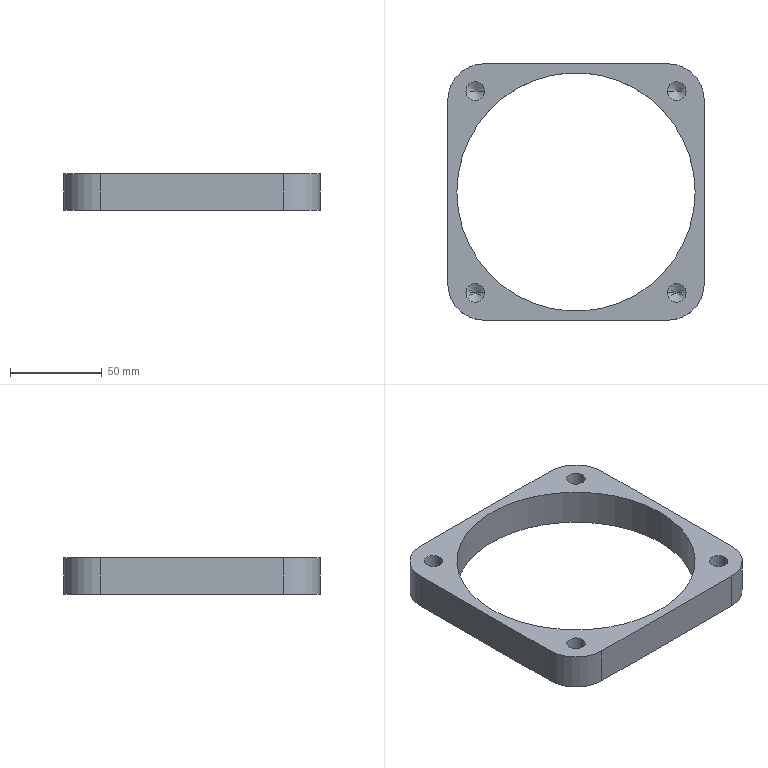Part | SolidWorks | features 3DProfileFeature 1, Extrusion 1, HoleWzd 1 | 1 solid | 28 faces | box 140 x 140 x 20 mm | volume 114105 mm3 | cylinder 14 | cone 8 | plane 6 | commonest cylinder face diameters 10.2 x8 40 x4 130 x2
STEP:
#1=CARTESIAN_POINT('',(9.9,125.,4.));
#2=VERTEX_POINT('',#1);
#3=CARTESIAN_POINT('',(20.1,125.,4.));
#4=VERTEX_POINT('',#3);
#5=CARTESIAN_POINT('',(15.,125.,4.));
#6=DIRECTION('',(0.,0.,1.));
#7=DIRECTION('',(1.,0.,0.));
#8=AXIS2_PLACEMENT_3D('',#5,#6,#7);
#9=CIRCLE('',#8,5.1);
#10=EDGE_CURVE('',#2,#4,#9,.T.);
#11=ORIENTED_EDGE('',*,*,#10,.F.);
#12=CARTESIAN_POINT('',(9.9,125.,20.));
#13=VERTEX_POINT('',#12);
#14=CARTESIAN_POINT('',(9.9,125.,20.));
#15=DIRECTION('',(0.,0.,1.));
#16=VECTOR('',#15,1000.);
#17=LINE('',#14,#16);
#18=EDGE_CURVE('',#2,#13,#17,.T.);
#19=ORIENTED_EDGE('',*,*,#18,.T.);
#20=CARTESIAN_POINT('',(20.1,125.,20.));
#21=VERTEX_POINT('',#20);
#22=CARTESIAN_POINT('',(15.,125.,20.));
#23=DIRECTION('',(0.,0.,1.));
#24=DIRECTION('',(1.,0.,0.));
#25=AXIS2_PLACEMENT_3D('',#22,#23,#24);
#26=CIRCLE('',#25,5.1);
#27=EDGE_CURVE('',#13,#21,#26,.T.);
#28=ORIENTED_EDGE('',*,*,#27,.T.);
#29=CARTESIAN_POINT('',(20.1,125.,20.));
#30=DIRECTION('',(0.,0.,1.));
#31=VECTOR('',#30,1000.);
#32=LINE('',#29,#31);
#33=EDGE_CURVE('',#4,#21,#32,.T.);
#34=ORIENTED_EDGE('',*,*,#33,.F.);
#35=EDGE_LOOP('',(#11,#19,#28,#34));
#36=FACE_OUTER_BOUND('',#35,.T.);
#37=CARTESIAN_POINT('',(15.,125.,20.));
#38=DIRECTION('',(0.,0.,1.));
#39=DIRECTION('',(1.,0.,0.));
#40=AXIS2_PLACEMENT_3D('',#37,#38,#39);
#41=CYLINDRICAL_SURFACE('',#40,5.1);
#42=ADVANCED_FACE('',(#36),#41,.F.);
#43=CARTESIAN_POINT('',(15.,125.,0.9356));
#44=VERTEX_POINT('',#43);
#45=CARTESIAN_POINT('',(20.1,125.,4.));
#46=DIRECTION('',(0.8572,0.,0.515));
#47=VECTOR('',#46,1000.);
#48=LINE('',#45,#47);
#49=EDGE_CURVE('',#44,#4,#48,.T.);
#50=ORIENTED_EDGE('',*,*,#49,.F.);
#51=CARTESIAN_POINT('',(9.9,125.,4.));
#52=DIRECTION('',(-0.8572,0.,0.515));
#53=VECTOR('',#52,1000.);
#54=LINE('',#51,#53);
#55=EDGE_CURVE('',#44,#2,#54,.T.);
#56=ORIENTED_EDGE('',*,*,#55,.T.);
#57=ORIENTED_EDGE('',*,*,#10,.T.);
#58=EDGE_LOOP('',(#50,#56,#57));
#59=FACE_OUTER_BOUND('',#58,.T.);
#60=CARTESIAN_POINT('',(15.,125.,4.));
#61=DIRECTION('',(0.,0.,1.));
#62=DIRECTION('',(1.,0.,0.));
#63=AXIS2_PLACEMENT_3D('',#60,#61,#62);
#64=CONICAL_SURFACE('',#63,5.1,1.03);
#65=ADVANCED_FACE('',(#59),#64,.F.);
#66=CARTESIAN_POINT('',(119.9,125.,4.));
#67=VERTEX_POINT('',#66);
#68=CARTESIAN_POINT('',(130.1,125.,4.));
#69=VERTEX_POINT('',#68);
#70=CARTESIAN_POINT('',(125.,125.,4.));
#71=DIRECTION('',(0.,0.,1.));
#72=DIRECTION('',(1.,0.,0.));
#73=AXIS2_PLACEMENT_3D('',#70,#71,#72);
#74=CIRCLE('',#73,5.1);
#75=EDGE_CURVE('',#67,#69,#74,.T.);
#76=ORIENTED_EDGE('',*,*,#75,.F.);
#77=CARTESIAN_POINT('',(119.9,125.,20.));
#78=VERTEX_POINT('',#77);
#79=CARTESIAN_POINT('',(119.9,125.,20.));
#80=DIRECTION('',(0.,0.,1.));
#81=VECTOR('',#80,1000.);
#82=LINE('',#79,#81);
#83=EDGE_CURVE('',#67,#78,#82,.T.);
#84=ORIENTED_EDGE('',*,*,#83,.T.);
#85=CARTESIAN_POINT('',(130.1,125.,20.));
#86=VERTEX_POINT('',#85);
#87=CARTESIAN_POINT('',(125.,125.,20.));
#88=DIRECTION('',(0.,0.,1.));
#89=DIRECTION('',(1.,0.,0.));
#90=AXIS2_PLACEMENT_3D('',#87,#88,#89);
#91=CIRCLE('',#90,5.1);
#92=EDGE_CURVE('',#78,#86,#91,.T.);
#93=ORIENTED_EDGE('',*,*,#92,.T.);
#94=CARTESIAN_POINT('',(130.1,125.,20.));
#95=DIRECTION('',(0.,0.,1.));
#96=VECTOR('',#95,1000.);
#97=LINE('',#94,#96);
#98=EDGE_CURVE('',#69,#86,#97,.T.);
#99=ORIENTED_EDGE('',*,*,#98,.F.);
#100=EDGE_LOOP('',(#76,#84,#93,#99));
#101=FACE_OUTER_BOUND('',#100,.T.);
#102=CARTESIAN_POINT('',(125.,125.,20.));
#103=DIRECTION('',(0.,0.,1.));
#104=DIRECTION('',(1.,0.,0.));
#105=AXIS2_PLACEMENT_3D('',#102,#103,#104);
#106=CYLINDRICAL_SURFACE('',#105,5.1);
#107=ADVANCED_FACE('',(#101),#106,.F.);
#108=CARTESIAN_POINT('',(125.,125.,0.9356));
#109=VERTEX_POINT('',#108);
#110=CARTESIAN_POINT('',(130.1,125.,4.));
#111=DIRECTION('',(0.8572,0.,0.515));
#112=VECTOR('',#111,1000.);
#113=LINE('',#110,#112);
#114=EDGE_CURVE('',#109,#69,#113,.T.);
#115=ORIENTED_EDGE('',*,*,#114,.F.);
#116=CARTESIAN_POINT('',(119.9,125.,4.));
#117=DIRECTION('',(-0.8572,0.,0.515));
#118=VECTOR('',#117,1000.);
#119=LINE('',#116,#118);
#120=EDGE_CURVE('',#109,#67,#119,.T.);
#121=ORIENTED_EDGE('',*,*,#120,.T.);
#122=ORIENTED_EDGE('',*,*,#75,.T.);
#123=EDGE_LOOP('',(#115,#121,#122));
#124=FACE_OUTER_BOUND('',#123,.T.);
#125=CARTESIAN_POINT('',(125.,125.,4.));
#126=DIRECTION('',(0.,0.,1.));
#127=DIRECTION('',(1.,0.,0.));
#128=AXIS2_PLACEMENT_3D('',#125,#126,#127);
#129=CONICAL_SURFACE('',#128,5.1,1.03);
#130=ADVANCED_FACE('',(#124),#129,.F.);
#131=CARTESIAN_POINT('',(119.9,15.,4.));
#132=VERTEX_POINT('',#131);
#133=CARTESIAN_POINT('',(130.1,15.,4.));
#134=VERTEX_POINT('',#133);
#135=CARTESIAN_POINT('',(125.,15.,4.));
#136=DIRECTION('',(0.,0.,1.));
#137=DIRECTION('',(1.,0.,0.));
#138=AXIS2_PLACEMENT_3D('',#135,#136,#137);
#139=CIRCLE('',#138,5.1);
#140=EDGE_CURVE('',#132,#134,#139,.T.);
#141=ORIENTED_EDGE('',*,*,#140,.F.);
#142=CARTESIAN_POINT('',(119.9,15.,20.));
#143=VERTEX_POINT('',#142);
#144=CARTESIAN_POINT('',(119.9,15.,20.));
#145=DIRECTION('',(0.,0.,1.));
#146=VECTOR('',#145,1000.);
#147=LINE('',#144,#146);
#148=EDGE_CURVE('',#132,#143,#147,.T.);
#149=ORIENTED_EDGE('',*,*,#148,.T.);
#150=CARTESIAN_POINT('',(130.1,15.,20.));
#151=VERTEX_POINT('',#150);
#152=CARTESIAN_POINT('',(125.,15.,20.));
#153=DIRECTION('',(0.,0.,1.));
#154=DIRECTION('',(1.,0.,0.));
#155=AXIS2_PLACEMENT_3D('',#152,#153,#154);
#156=CIRCLE('',#155,5.1);
#157=EDGE_CURVE('',#143,#151,#156,.T.);
#158=ORIENTED_EDGE('',*,*,#157,.T.);
#159=CARTESIAN_POINT('',(130.1,15.,20.));
#160=DIRECTION('',(0.,0.,1.));
#161=VECTOR('',#160,1000.);
#162=LINE('',#159,#161);
#163=EDGE_CURVE('',#134,#151,#162,.T.);
#164=ORIENTED_EDGE('',*,*,#163,.F.);
#165=EDGE_LOOP('',(#141,#149,#158,#164));
#166=FACE_OUTER_BOUND('',#165,.T.);
#167=CARTESIAN_POINT('',(125.,15.,20.));
#168=DIRECTION('',(0.,0.,1.));
#169=DIRECTION('',(1.,0.,0.));
#170=AXIS2_PLACEMENT_3D('',#167,#168,#169);
#171=CYLINDRICAL_SURFACE('',#170,5.1);
#172=ADVANCED_FACE('',(#166),#171,.F.);
#173=CARTESIAN_POINT('',(125.,15.,0.9356));
#174=VERTEX_POINT('',#173);
#175=CARTESIAN_POINT('',(130.1,15.,4.));
#176=DIRECTION('',(0.8572,0.,0.515));
#177=VECTOR('',#176,1000.);
#178=LINE('',#175,#177);
#179=EDGE_CURVE('',#174,#134,#178,.T.);
#180=ORIENTED_EDGE('',*,*,#179,.F.);
#181=CARTESIAN_POINT('',(119.9,15.,4.));
#182=DIRECTION('',(-0.8572,0.,0.515));
#183=VECTOR('',#182,1000.);
#184=LINE('',#181,#183);
#185=EDGE_CURVE('',#174,#132,#184,.T.);
#186=ORIENTED_EDGE('',*,*,#185,.T.);
#187=ORIENTED_EDGE('',*,*,#140,.T.);
#188=EDGE_LOOP('',(#180,#186,#187));
#189=FACE_OUTER_BOUND('',#188,.T.);
#190=CARTESIAN_POINT('',(125.,15.,4.));
#191=DIRECTION('',(0.,0.,1.));
#192=DIRECTION('',(1.,0.,0.));
#193=AXIS2_PLACEMENT_3D('',#190,#191,#192);
#194=CONICAL_SURFACE('',#193,5.1,1.03);
#195=ADVANCED_FACE('',(#189),#194,.F.);
#196=CARTESIAN_POINT('',(9.9,15.,4.));
#197=VERTEX_POINT('',#196);
#198=CARTESIAN_POINT('',(20.1,15.,4.));
#199=VERTEX_POINT('',#198);
#200=CARTESIAN_POINT('',(15.,15.,4.));
#201=DIRECTION('',(0.,0.,1.));
#202=DIRECTION('',(1.,0.,0.));
#203=AXIS2_PLACEMENT_3D('',#200,#201,#202);
#204=CIRCLE('',#203,5.1);
#205=EDGE_CURVE('',#197,#199,#204,.T.);
#206=ORIENTED_EDGE('',*,*,#205,.F.);
#207=CARTESIAN_POINT('',(9.9,15.,20.));
#208=VERTEX_POINT('',#207);
#209=CARTESIAN_POINT('',(9.9,15.,20.));
#210=DIRECTION('',(0.,0.,1.));
#211=VECTOR('',#210,1000.);
#212=LINE('',#209,#211);
#213=EDGE_CURVE('',#197,#208,#212,.T.);
#214=ORIENTED_EDGE('',*,*,#213,.T.);
#215=CARTESIAN_POINT('',(20.1,15.,20.));
#216=VERTEX_POINT('',#215);
#217=CARTESIAN_POINT('',(15.,15.,20.));
#218=DIRECTION('',(0.,0.,1.));
#219=DIRECTION('',(1.,0.,0.));
#220=AXIS2_PLACEMENT_3D('',#217,#218,#219);
#221=CIRCLE('',#220,5.1);
#222=EDGE_CURVE('',#208,#216,#221,.T.);
#223=ORIENTED_EDGE('',*,*,#222,.T.);
#224=CARTESIAN_POINT('',(20.1,15.,20.));
#225=DIRECTION('',(0.,0.,1.));
#226=VECTOR('',#225,1000.);
#227=LINE('',#224,#226);
#228=EDGE_CURVE('',#199,#216,#227,.T.);
#229=ORIENTED_EDGE('',*,*,#228,.F.);
#230=EDGE_LOOP('',(#206,#214,#223,#229));
#231=FACE_OUTER_BOUND('',#230,.T.);
#232=CARTESIAN_POINT('',(15.,15.,20.));
#233=DIRECTION('',(0.,0.,1.));
#234=DIRECTION('',(1.,0.,0.));
#235=AXIS2_PLACEMENT_3D('',#232,#233,#234);
#236=CYLINDRICAL_SURFACE('',#235,5.1);
#237=ADVANCED_FACE('',(#231),#236,.F.);
#238=CARTESIAN_POINT('',(15.,15.,0.9356));
#239=VERTEX_POINT('',#238);
#240=CARTESIAN_POINT('',(20.1,15.,4.));
#241=DIRECTION('',(0.8572,0.,0.515));
#242=VECTOR('',#241,1000.);
#243=LINE('',#240,#242);
#244=EDGE_CURVE('',#239,#199,#243,.T.);
#245=ORIENTED_EDGE('',*,*,#244,.F.);
#246=CARTESIAN_POINT('',(9.9,15.,4.));
#247=DIRECTION('',(-0.8572,0.,0.515));
#248=VECTOR('',#247,1000.);
#249=LINE('',#246,#248);
#250=EDGE_CURVE('',#239,#197,#249,.T.);
#251=ORIENTED_EDGE('',*,*,#250,.T.);
#252=ORIENTED_EDGE('',*,*,#205,.T.);
#253=EDGE_LOOP('',(#245,#251,#252));
#254=FACE_OUTER_BOUND('',#253,.T.);
#255=CARTESIAN_POINT('',(15.,15.,4.));
#256=DIRECTION('',(0.,0.,1.));
#257=DIRECTION('',(1.,0.,0.));
#258=AXIS2_PLACEMENT_3D('',#255,#256,#257);
#259=CONICAL_SURFACE('',#258,5.1,1.03);
#260=ADVANCED_FACE('',(#254),#259,.F.);
#261=CARTESIAN_POINT('',(5.,70.,20.));
#262=VERTEX_POINT('',#261);
#263=CARTESIAN_POINT('',(135.,70.,20.));
#264=VERTEX_POINT('',#263);
#265=CARTESIAN_POINT('',(70.,70.,20.));
#266=DIRECTION('',(0.,0.,1.));
#267=DIRECTION('',(1.,0.,0.));
#268=AXIS2_PLACEMENT_3D('',#265,#266,#267);
#269=CIRCLE('',#268,65.);
#270=EDGE_CURVE('',#262,#264,#269,.T.);
#271=ORIENTED_EDGE('',*,*,#270,.T.);
#272=CARTESIAN_POINT('',(135.,70.,0.));
#273=VERTEX_POINT('',#272);
#274=CARTESIAN_POINT('',(135.,70.,20.));
#275=DIRECTION('',(0.,0.,-1.));
#276=VECTOR('',#275,1000.);
#277=LINE('',#274,#276);
#278=EDGE_CURVE('',#264,#273,#277,.T.);
#279=ORIENTED_EDGE('',*,*,#278,.T.);
#280=CARTESIAN_POINT('',(5.,70.,0.));
#281=VERTEX_POINT('',#280);
#282=CARTESIAN_POINT('',(70.,70.,0.));
#283=DIRECTION('',(0.,0.,1.));
#284=DIRECTION('',(1.,0.,0.));
#285=AXIS2_PLACEMENT_3D('',#282,#283,#284);
#286=CIRCLE('',#285,65.);
#287=EDGE_CURVE('',#281,#273,#286,.T.);
#288=ORIENTED_EDGE('',*,*,#287,.F.);
#289=CARTESIAN_POINT('',(5.,70.,20.));
#290=DIRECTION('',(0.,0.,-1.));
#291=VECTOR('',#290,1000.);
#292=LINE('',#289,#291);
#293=EDGE_CURVE('',#262,#281,#292,.T.);
#294=ORIENTED_EDGE('',*,*,#293,.F.);
#295=EDGE_LOOP('',(#271,#279,#288,#294));
#296=FACE_OUTER_BOUND('',#295,.T.);
#297=CARTESIAN_POINT('',(70.,70.,20.));
#298=DIRECTION('',(0.,0.,-1.));
#299=DIRECTION('',(-1.,0.,0.));
#300=AXIS2_PLACEMENT_3D('',#297,#298,#299);
#301=CYLINDRICAL_SURFACE('',#300,65.);
#302=ADVANCED_FACE('',(#296),#301,.F.);
#303=CARTESIAN_POINT('',(15.,125.,20.));
#304=DIRECTION('',(0.,0.,1.));
#305=DIRECTION('',(1.,0.,0.));
#306=AXIS2_PLACEMENT_3D('',#303,#304,#305);
#307=CIRCLE('',#306,5.1);
#308=EDGE_CURVE('',#21,#13,#307,.T.);
#309=ORIENTED_EDGE('',*,*,#308,.F.);
#310=ORIENTED_EDGE('',*,*,#27,.F.);
#311=EDGE_LOOP('',(#309,#310));
#312=FACE_BOUND('',#311,.T.);
#313=CARTESIAN_POINT('',(125.,125.,20.));
#314=DIRECTION('',(0.,0.,1.));
#315=DIRECTION('',(1.,0.,0.));
#316=AXIS2_PLACEMENT_3D('',#313,#314,#315);
#317=CIRCLE('',#316,5.1);
#318=EDGE_CURVE('',#86,#78,#317,.T.);
#319=ORIENTED_EDGE('',*,*,#318,.F.);
#320=ORIENTED_EDGE('',*,*,#92,.F.);
#321=EDGE_LOOP('',(#319,#320));
#322=FACE_BOUND('',#321,.T.);
#323=CARTESIAN_POINT('',(125.,15.,20.));
#324=DIRECTION('',(0.,0.,1.));
#325=DIRECTION('',(1.,0.,0.));
#326=AXIS2_PLACEMENT_3D('',#323,#324,#325);
#327=CIRCLE('',#326,5.1);
#328=EDGE_CURVE('',#151,#143,#327,.T.);
#329=ORIENTED_EDGE('',*,*,#328,.F.);
#330=ORIENTED_EDGE('',*,*,#157,.F.);
#331=EDGE_LOOP('',(#329,#330));
#332=FACE_BOUND('',#331,.T.);
#333=CARTESIAN_POINT('',(15.,15.,20.));
#334=DIRECTION('',(0.,0.,1.));
#335=DIRECTION('',(1.,0.,0.));
#336=AXIS2_PLACEMENT_3D('',#333,#334,#335);
#337=CIRCLE('',#336,5.1);
#338=EDGE_CURVE('',#216,#208,#337,.T.);
#339=ORIENTED_EDGE('',*,*,#338,.F.);
#340=ORIENTED_EDGE('',*,*,#222,.F.);
#341=EDGE_LOOP('',(#339,#340));
#342=FACE_BOUND('',#341,.T.);
#343=CARTESIAN_POINT('',(0.,20.,20.));
#344=VERTEX_POINT('',#343);
#345=CARTESIAN_POINT('',(20.,0.,20.));
#346=VERTEX_POINT('',#345);
#347=CARTESIAN_POINT('',(20.,20.,20.));
#348=DIRECTION('',(0.,0.,1.));
#349=DIRECTION('',(-1.,0.,0.));
#350=AXIS2_PLACEMENT_3D('',#347,#348,#349);
#351=CIRCLE('',#350,20.);
#352=EDGE_CURVE('',#344,#346,#351,.T.);
#353=ORIENTED_EDGE('',*,*,#352,.T.);
#354=CARTESIAN_POINT('',(120.,0.,20.));
#355=VERTEX_POINT('',#354);
#356=CARTESIAN_POINT('',(20.,0.,20.));
#357=DIRECTION('',(1.,0.,0.));
#358=VECTOR('',#357,1000.);
#359=LINE('',#356,#358);
#360=EDGE_CURVE('',#346,#355,#359,.T.);
#361=ORIENTED_EDGE('',*,*,#360,.T.);
#362=CARTESIAN_POINT('',(140.,20.,20.));
#363=VERTEX_POINT('',#362);
#364=CARTESIAN_POINT('',(120.,20.,20.));
#365=DIRECTION('',(0.,0.,1.));
#366=DIRECTION('',(1.,0.,0.));
#367=AXIS2_PLACEMENT_3D('',#364,#365,#366);
#368=CIRCLE('',#367,20.);
#369=EDGE_CURVE('',#355,#363,#368,.T.);
#370=ORIENTED_EDGE('',*,*,#369,.T.);
#371=CARTESIAN_POINT('',(140.,120.,20.));
#372=VERTEX_POINT('',#371);
#373=CARTESIAN_POINT('',(140.,20.,20.));
#374=DIRECTION('',(0.,1.,0.));
#375=VECTOR('',#374,1000.);
#376=LINE('',#373,#375);
#377=EDGE_CURVE('',#363,#372,#376,.T.);
#378=ORIENTED_EDGE('',*,*,#377,.T.);
#379=CARTESIAN_POINT('',(120.,140.,20.));
#380=VERTEX_POINT('',#379);
#381=CARTESIAN_POINT('',(120.,120.,20.));
#382=DIRECTION('',(0.,0.,1.));
#383=DIRECTION('',(-1.,0.,0.));
#384=AXIS2_PLACEMENT_3D('',#381,#382,#383);
#385=CIRCLE('',#384,20.);
#386=EDGE_CURVE('',#372,#380,#385,.T.);
#387=ORIENTED_EDGE('',*,*,#386,.T.);
#388=CARTESIAN_POINT('',(20.,140.,20.));
#389=VERTEX_POINT('',#388);
#390=CARTESIAN_POINT('',(20.,140.,20.));
#391=DIRECTION('',(-1.,0.,0.));
#392=VECTOR('',#391,1000.);
#393=LINE('',#390,#392);
#394=EDGE_CURVE('',#380,#389,#393,.T.);
#395=ORIENTED_EDGE('',*,*,#394,.T.);
#396=CARTESIAN_POINT('',(0.,120.,20.));
#397=VERTEX_POINT('',#396);
#398=CARTESIAN_POINT('',(20.,120.,20.));
#399=DIRECTION('',(0.,0.,1.));
#400=DIRECTION('',(-1.,0.,0.));
#401=AXIS2_PLACEMENT_3D('',#398,#399,#400);
#402=CIRCLE('',#401,20.);
#403=EDGE_CURVE('',#389,#397,#402,.T.);
#404=ORIENTED_EDGE('',*,*,#403,.T.);
#405=CARTESIAN_POINT('',(0.,20.,20.));
#406=DIRECTION('',(0.,-1.,0.));
#407=VECTOR('',#406,1000.);
#408=LINE('',#405,#407);
#409=EDGE_CURVE('',#397,#344,#408,.T.);
#410=ORIENTED_EDGE('',*,*,#409,.T.);
#411=EDGE_LOOP('',(#353,#361,#370,#378,#387,#395,#404,#410));
#412=FACE_OUTER_BOUND('',#411,.T.);
#413=ORIENTED_EDGE('',*,*,#270,.F.);
#414=CARTESIAN_POINT('',(70.,70.,20.));
#415=DIRECTION('',(0.,0.,1.));
#416=DIRECTION('',(1.,0.,0.));
#417=AXIS2_PLACEMENT_3D('',#414,#415,#416);
#418=CIRCLE('',#417,65.);
#419=EDGE_CURVE('',#264,#262,#418,.T.);
#420=ORIENTED_EDGE('',*,*,#419,.F.);
#421=EDGE_LOOP('',(#413,#420));
#422=FACE_BOUND('',#421,.T.);
#423=CARTESIAN_POINT('',(20.,20.,20.));
#424=DIRECTION('',(0.,0.,-1.));
#425=DIRECTION('',(-1.,0.,0.));
#426=AXIS2_PLACEMENT_3D('',#423,#424,#425);
#427=PLANE('',#426);
#428=ADVANCED_FACE('',(#312,#322,#332,#342,#412,#422),#427,.F.);
#429=CARTESIAN_POINT('',(0.,20.,0.));
#430=VERTEX_POINT('',#429);
#431=CARTESIAN_POINT('',(20.,0.,0.));
#432=VERTEX_POINT('',#431);
#433=CARTESIAN_POINT('',(20.,20.,0.));
#434=DIRECTION('',(0.,0.,1.));
#435=DIRECTION('',(-1.,0.,0.));
#436=AXIS2_PLACEMENT_3D('',#433,#434,#435);
#437=CIRCLE('',#436,20.);
#438=EDGE_CURVE('',#430,#432,#437,.T.);
#439=ORIENTED_EDGE('',*,*,#438,.F.);
#440=CARTESIAN_POINT('',(0.,120.,0.));
#441=VERTEX_POINT('',#440);
#442=CARTESIAN_POINT('',(0.,20.,0.));
#443=DIRECTION('',(0.,-1.,0.));
#444=VECTOR('',#443,1000.);
#445=LINE('',#442,#444);
#446=EDGE_CURVE('',#441,#430,#445,.T.);
#447=ORIENTED_EDGE('',*,*,#446,.F.);
#448=CARTESIAN_POINT('',(20.,140.,0.));
#449=VERTEX_POINT('',#448);
#450=CARTESIAN_POINT('',(20.,120.,0.));
#451=DIRECTION('',(0.,0.,1.));
#452=DIRECTION('',(-1.,0.,0.));
#453=AXIS2_PLACEMENT_3D('',#450,#451,#452);
#454=CIRCLE('',#453,20.);
#455=EDGE_CURVE('',#449,#441,#454,.T.);
#456=ORIENTED_EDGE('',*,*,#455,.F.);
#457=CARTESIAN_POINT('',(120.,140.,0.));
#458=VERTEX_POINT('',#457);
#459=CARTESIAN_POINT('',(20.,140.,0.));
#460=DIRECTION('',(-1.,0.,0.));
#461=VECTOR('',#460,1000.);
#462=LINE('',#459,#461);
#463=EDGE_CURVE('',#458,#449,#462,.T.);
#464=ORIENTED_EDGE('',*,*,#463,.F.);
#465=CARTESIAN_POINT('',(140.,120.,0.));
#466=VERTEX_POINT('',#465);
#467=CARTESIAN_POINT('',(120.,120.,0.));
#468=DIRECTION('',(0.,0.,1.));
#469=DIRECTION('',(-1.,0.,0.));
#470=AXIS2_PLACEMENT_3D('',#467,#468,#469);
#471=CIRCLE('',#470,20.);
#472=EDGE_CURVE('',#466,#458,#471,.T.);
#473=ORIENTED_EDGE('',*,*,#472,.F.);
#474=CARTESIAN_POINT('',(140.,20.,0.));
#475=VERTEX_POINT('',#474);
#476=CARTESIAN_POINT('',(140.,20.,0.));
#477=DIRECTION('',(0.,1.,0.));
#478=VECTOR('',#477,1000.);
#479=LINE('',#476,#478);
#480=EDGE_CURVE('',#475,#466,#479,.T.);
#481=ORIENTED_EDGE('',*,*,#480,.F.);
#482=CARTESIAN_POINT('',(120.,0.,0.));
#483=VERTEX_POINT('',#482);
#484=CARTESIAN_POINT('',(120.,20.,0.));
#485=DIRECTION('',(0.,0.,1.));
#486=DIRECTION('',(1.,0.,0.));
#487=AXIS2_PLACEMENT_3D('',#484,#485,#486);
#488=CIRCLE('',#487,20.);
#489=EDGE_CURVE('',#483,#475,#488,.T.);
#490=ORIENTED_EDGE('',*,*,#489,.F.);
#491=CARTESIAN_POINT('',(20.,0.,0.));
#492=DIRECTION('',(1.,0.,0.));
#493=VECTOR('',#492,1000.);
#494=LINE('',#491,#493);
#495=EDGE_CURVE('',#432,#483,#494,.T.);
#496=ORIENTED_EDGE('',*,*,#495,.F.);
#497=EDGE_LOOP('',(#439,#447,#456,#464,#473,#481,#490,#496));
#498=FACE_OUTER_BOUND('',#497,.T.);
#499=ORIENTED_EDGE('',*,*,#287,.T.);
#500=CARTESIAN_POINT('',(70.,70.,0.));
#501=DIRECTION('',(0.,0.,1.));
#502=DIRECTION('',(1.,0.,0.));
#503=AXIS2_PLACEMENT_3D('',#500,#501,#502);
#504=CIRCLE('',#503,65.);
#505=EDGE_CURVE('',#273,#281,#504,.T.);
#506=ORIENTED_EDGE('',*,*,#505,.T.);
#507=EDGE_LOOP('',(#499,#506));
#508=FACE_BOUND('',#507,.T.);
#509=CARTESIAN_POINT('',(20.,20.,0.));
#510=DIRECTION('',(0.,0.,-1.));
#511=DIRECTION('',(-1.,0.,0.));
#512=AXIS2_PLACEMENT_3D('',#509,#510,#511);
#513=PLANE('',#512);
#514=ADVANCED_FACE('',(#498,#508),#513,.T.);
#515=ORIENTED_EDGE('',*,*,#438,.T.);
#516=CARTESIAN_POINT('',(20.,0.,20.));
#517=DIRECTION('',(0.,0.,-1.));
#518=VECTOR('',#517,1000.);
#519=LINE('',#516,#518);
#520=EDGE_CURVE('',#346,#432,#519,.T.);
#521=ORIENTED_EDGE('',*,*,#520,.F.);
#522=ORIENTED_EDGE('',*,*,#352,.F.);
#523=CARTESIAN_POINT('',(0.,20.,20.));
#524=DIRECTION('',(0.,0.,-1.));
#525=VECTOR('',#524,1000.);
#526=LINE('',#523,#525);
#527=EDGE_CURVE('',#344,#430,#526,.T.);
#528=ORIENTED_EDGE('',*,*,#527,.T.);
#529=EDGE_LOOP('',(#515,#521,#522,#528));
#530=FACE_OUTER_BOUND('',#529,.T.);
#531=CARTESIAN_POINT('',(20.,20.,20.));
#532=DIRECTION('',(0.,0.,-1.));
#533=DIRECTION('',(-1.,0.,0.));
#534=AXIS2_PLACEMENT_3D('',#531,#532,#533);
#535=CYLINDRICAL_SURFACE('',#534,20.);
#536=ADVANCED_FACE('',(#530),#535,.T.);
#537=ORIENTED_EDGE('',*,*,#495,.T.);
#538=CARTESIAN_POINT('',(120.,0.,20.));
#539=DIRECTION('',(0.,0.,-1.));
#540=VECTOR('',#539,1000.);
#541=LINE('',#538,#540);
#542=EDGE_CURVE('',#355,#483,#541,.T.);
#543=ORIENTED_EDGE('',*,*,#542,.F.);
#544=ORIENTED_EDGE('',*,*,#360,.F.);
#545=ORIENTED_EDGE('',*,*,#520,.T.);
#546=EDGE_LOOP('',(#537,#543,#544,#545));
#547=FACE_OUTER_BOUND('',#546,.T.);
#548=CARTESIAN_POINT('',(20.,0.,20.));
#549=DIRECTION('',(0.,1.,0.));
#550=DIRECTION('',(0.,0.,1.));
#551=AXIS2_PLACEMENT_3D('',#548,#549,#550);
#552=PLANE('',#551);
#553=ADVANCED_FACE('',(#547),#552,.F.);
#554=ORIENTED_EDGE('',*,*,#489,.T.);
#555=CARTESIAN_POINT('',(140.,20.,20.));
#556=DIRECTION('',(0.,0.,-1.));
#557=VECTOR('',#556,1000.);
#558=LINE('',#555,#557);
#559=EDGE_CURVE('',#363,#475,#558,.T.);
#560=ORIENTED_EDGE('',*,*,#559,.F.);
#561=ORIENTED_EDGE('',*,*,#369,.F.);
#562=ORIENTED_EDGE('',*,*,#542,.T.);
#563=EDGE_LOOP('',(#554,#560,#561,#562));
#564=FACE_OUTER_BOUND('',#563,.T.);
#565=CARTESIAN_POINT('',(120.,20.,20.));
#566=DIRECTION('',(0.,0.,-1.));
#567=DIRECTION('',(-1.,0.,0.));
#568=AXIS2_PLACEMENT_3D('',#565,#566,#567);
#569=CYLINDRICAL_SURFACE('',#568,20.);
#570=ADVANCED_FACE('',(#564),#569,.T.);
#571=ORIENTED_EDGE('',*,*,#480,.T.);
#572=CARTESIAN_POINT('',(140.,120.,20.));
#573=DIRECTION('',(0.,0.,-1.));
#574=VECTOR('',#573,1000.);
#575=LINE('',#572,#574);
#576=EDGE_CURVE('',#372,#466,#575,.T.);
#577=ORIENTED_EDGE('',*,*,#576,.F.);
#578=ORIENTED_EDGE('',*,*,#377,.F.);
#579=ORIENTED_EDGE('',*,*,#559,.T.);
#580=EDGE_LOOP('',(#571,#577,#578,#579));
#581=FACE_OUTER_BOUND('',#580,.T.);
#582=CARTESIAN_POINT('',(140.,20.,20.));
#583=DIRECTION('',(-1.,0.,0.));
#584=DIRECTION('',(0.,0.,1.));
#585=AXIS2_PLACEMENT_3D('',#582,#583,#584);
#586=PLANE('',#585);
#587=ADVANCED_FACE('',(#581),#586,.F.);
#588=ORIENTED_EDGE('',*,*,#472,.T.);
#589=CARTESIAN_POINT('',(120.,140.,20.));
#590=DIRECTION('',(0.,0.,-1.));
#591=VECTOR('',#590,1000.);
#592=LINE('',#589,#591);
#593=EDGE_CURVE('',#380,#458,#592,.T.);
#594=ORIENTED_EDGE('',*,*,#593,.F.);
#595=ORIENTED_EDGE('',*,*,#386,.F.);
#596=ORIENTED_EDGE('',*,*,#576,.T.);
#597=EDGE_LOOP('',(#588,#594,#595,#596));
#598=FACE_OUTER_BOUND('',#597,.T.);
#599=CARTESIAN_POINT('',(120.,120.,20.));
#600=DIRECTION('',(0.,0.,-1.));
#601=DIRECTION('',(-1.,0.,0.));
#602=AXIS2_PLACEMENT_3D('',#599,#600,#601);
#603=CYLINDRICAL_SURFACE('',#602,20.);
#604=ADVANCED_FACE('',(#598),#603,.T.);
#605=ORIENTED_EDGE('',*,*,#463,.T.);
#606=CARTESIAN_POINT('',(20.,140.,20.));
#607=DIRECTION('',(0.,0.,-1.));
#608=VECTOR('',#607,1000.);
#609=LINE('',#606,#608);
#610=EDGE_CURVE('',#389,#449,#609,.T.);
#611=ORIENTED_EDGE('',*,*,#610,.F.);
#612=ORIENTED_EDGE('',*,*,#394,.F.);
#613=ORIENTED_EDGE('',*,*,#593,.T.);
#614=EDGE_LOOP('',(#605,#611,#612,#613));
#615=FACE_OUTER_BOUND('',#614,.T.);
#616=CARTESIAN_POINT('',(20.,140.,20.));
#617=DIRECTION('',(0.,-1.,0.));
#618=DIRECTION('',(0.,0.,-1.));
#619=AXIS2_PLACEMENT_3D('',#616,#617,#618);
#620=PLANE('',#619);
#621=ADVANCED_FACE('',(#615),#620,.F.);
#622=ORIENTED_EDGE('',*,*,#455,.T.);
#623=CARTESIAN_POINT('',(0.,120.,20.));
#624=DIRECTION('',(0.,0.,-1.));
#625=VECTOR('',#624,1000.);
#626=LINE('',#623,#625);
#627=EDGE_CURVE('',#397,#441,#626,.T.);
#628=ORIENTED_EDGE('',*,*,#627,.F.);
#629=ORIENTED_EDGE('',*,*,#403,.F.);
#630=ORIENTED_EDGE('',*,*,#610,.T.);
#631=EDGE_LOOP('',(#622,#628,#629,#630));
#632=FACE_OUTER_BOUND('',#631,.T.);
#633=CARTESIAN_POINT('',(20.,120.,20.));
#634=DIRECTION('',(0.,0.,-1.));
#635=DIRECTION('',(-1.,0.,0.));
#636=AXIS2_PLACEMENT_3D('',#633,#634,#635);
#637=CYLINDRICAL_SURFACE('',#636,20.);
#638=ADVANCED_FACE('',(#632),#637,.T.);
#639=ORIENTED_EDGE('',*,*,#446,.T.);
#640=ORIENTED_EDGE('',*,*,#527,.F.);
#641=ORIENTED_EDGE('',*,*,#409,.F.);
#642=ORIENTED_EDGE('',*,*,#627,.T.);
#643=EDGE_LOOP('',(#639,#640,#641,#642));
#644=FACE_OUTER_BOUND('',#643,.T.);
#645=CARTESIAN_POINT('',(0.,20.,20.));
#646=DIRECTION('',(1.,0.,0.));
#647=DIRECTION('',(0.,0.,-1.));
#648=AXIS2_PLACEMENT_3D('',#645,#646,#647);
#649=PLANE('',#648);
#650=ADVANCED_FACE('',(#644),#649,.F.);
#651=ORIENTED_EDGE('',*,*,#278,.F.);
#652=ORIENTED_EDGE('',*,*,#419,.T.);
#653=ORIENTED_EDGE('',*,*,#293,.T.);
#654=ORIENTED_EDGE('',*,*,#505,.F.);
#655=EDGE_LOOP('',(#651,#652,#653,#654));
#656=FACE_OUTER_BOUND('',#655,.T.);
#657=CARTESIAN_POINT('',(70.,70.,20.));
#658=DIRECTION('',(0.,0.,-1.));
#659=DIRECTION('',(-1.,0.,0.));
#660=AXIS2_PLACEMENT_3D('',#657,#658,#659);
#661=CYLINDRICAL_SURFACE('',#660,65.);
#662=ADVANCED_FACE('',(#656),#661,.F.);
#663=ORIENTED_EDGE('',*,*,#250,.F.);
#664=ORIENTED_EDGE('',*,*,#244,.T.);
#665=CARTESIAN_POINT('',(15.,15.,4.));
#666=DIRECTION('',(0.,0.,1.));
#667=DIRECTION('',(1.,0.,0.));
#668=AXIS2_PLACEMENT_3D('',#665,#666,#667);
#669=CIRCLE('',#668,5.1);
#670=EDGE_CURVE('',#199,#197,#669,.T.);
#671=ORIENTED_EDGE('',*,*,#670,.T.);
#672=EDGE_LOOP('',(#663,#664,#671));
#673=FACE_OUTER_BOUND('',#672,.T.);
#674=CARTESIAN_POINT('',(15.,15.,4.));
#675=DIRECTION('',(0.,0.,1.));
#676=DIRECTION('',(1.,0.,0.));
#677=AXIS2_PLACEMENT_3D('',#674,#675,#676);
#678=CONICAL_SURFACE('',#677,5.1,1.03);
#679=ADVANCED_FACE('',(#673),#678,.F.);
#680=ORIENTED_EDGE('',*,*,#213,.F.);
#681=ORIENTED_EDGE('',*,*,#670,.F.);
#682=ORIENTED_EDGE('',*,*,#228,.T.);
#683=ORIENTED_EDGE('',*,*,#338,.T.);
#684=EDGE_LOOP('',(#680,#681,#682,#683));
#685=FACE_OUTER_BOUND('',#684,.T.);
#686=CARTESIAN_POINT('',(15.,15.,20.));
#687=DIRECTION('',(0.,0.,1.));
#688=DIRECTION('',(1.,0.,0.));
#689=AXIS2_PLACEMENT_3D('',#686,#687,#688);
#690=CYLINDRICAL_SURFACE('',#689,5.1);
#691=ADVANCED_FACE('',(#685),#690,.F.);
#692=ORIENTED_EDGE('',*,*,#185,.F.);
#693=ORIENTED_EDGE('',*,*,#179,.T.);
#694=CARTESIAN_POINT('',(125.,15.,4.));
#695=DIRECTION('',(0.,0.,1.));
#696=DIRECTION('',(1.,0.,0.));
#697=AXIS2_PLACEMENT_3D('',#694,#695,#696);
#698=CIRCLE('',#697,5.1);
#699=EDGE_CURVE('',#134,#132,#698,.T.);
#700=ORIENTED_EDGE('',*,*,#699,.T.);
#701=EDGE_LOOP('',(#692,#693,#700));
#702=FACE_OUTER_BOUND('',#701,.T.);
#703=CARTESIAN_POINT('',(125.,15.,4.));
#704=DIRECTION('',(0.,0.,1.));
#705=DIRECTION('',(1.,0.,0.));
#706=AXIS2_PLACEMENT_3D('',#703,#704,#705);
#707=CONICAL_SURFACE('',#706,5.1,1.03);
#708=ADVANCED_FACE('',(#702),#707,.F.);
#709=ORIENTED_EDGE('',*,*,#148,.F.);
#710=ORIENTED_EDGE('',*,*,#699,.F.);
#711=ORIENTED_EDGE('',*,*,#163,.T.);
#712=ORIENTED_EDGE('',*,*,#328,.T.);
#713=EDGE_LOOP('',(#709,#710,#711,#712));
#714=FACE_OUTER_BOUND('',#713,.T.);
#715=CARTESIAN_POINT('',(125.,15.,20.));
#716=DIRECTION('',(0.,0.,1.));
#717=DIRECTION('',(1.,0.,0.));
#718=AXIS2_PLACEMENT_3D('',#715,#716,#717);
#719=CYLINDRICAL_SURFACE('',#718,5.1);
#720=ADVANCED_FACE('',(#714),#719,.F.);
#721=ORIENTED_EDGE('',*,*,#120,.F.);
#722=ORIENTED_EDGE('',*,*,#114,.T.);
#723=CARTESIAN_POINT('',(125.,125.,4.));
#724=DIRECTION('',(0.,0.,1.));
#725=DIRECTION('',(1.,0.,0.));
#726=AXIS2_PLACEMENT_3D('',#723,#724,#725);
#727=CIRCLE('',#726,5.1);
#728=EDGE_CURVE('',#69,#67,#727,.T.);
#729=ORIENTED_EDGE('',*,*,#728,.T.);
#730=EDGE_LOOP('',(#721,#722,#729));
#731=FACE_OUTER_BOUND('',#730,.T.);
#732=CARTESIAN_POINT('',(125.,125.,4.));
#733=DIRECTION('',(0.,0.,1.));
#734=DIRECTION('',(1.,0.,0.));
#735=AXIS2_PLACEMENT_3D('',#732,#733,#734);
#736=CONICAL_SURFACE('',#735,5.1,1.03);
#737=ADVANCED_FACE('',(#731),#736,.F.);
#738=ORIENTED_EDGE('',*,*,#83,.F.);
#739=ORIENTED_EDGE('',*,*,#728,.F.);
#740=ORIENTED_EDGE('',*,*,#98,.T.);
#741=ORIENTED_EDGE('',*,*,#318,.T.);
#742=EDGE_LOOP('',(#738,#739,#740,#741));
#743=FACE_OUTER_BOUND('',#742,.T.);
#744=CARTESIAN_POINT('',(125.,125.,20.));
#745=DIRECTION('',(0.,0.,1.));
#746=DIRECTION('',(1.,0.,0.));
#747=AXIS2_PLACEMENT_3D('',#744,#745,#746);
#748=CYLINDRICAL_SURFACE('',#747,5.1);
#749=ADVANCED_FACE('',(#743),#748,.F.);
#750=ORIENTED_EDGE('',*,*,#55,.F.);
#751=ORIENTED_EDGE('',*,*,#49,.T.);
#752=CARTESIAN_POINT('',(15.,125.,4.));
#753=DIRECTION('',(0.,0.,1.));
#754=DIRECTION('',(1.,0.,0.));
#755=AXIS2_PLACEMENT_3D('',#752,#753,#754);
#756=CIRCLE('',#755,5.1);
#757=EDGE_CURVE('',#4,#2,#756,.T.);
#758=ORIENTED_EDGE('',*,*,#757,.T.);
#759=EDGE_LOOP('',(#750,#751,#758));
#760=FACE_OUTER_BOUND('',#759,.T.);
#761=CARTESIAN_POINT('',(15.,125.,4.));
#762=DIRECTION('',(0.,0.,1.));
#763=DIRECTION('',(1.,0.,0.));
#764=AXIS2_PLACEMENT_3D('',#761,#762,#763);
#765=CONICAL_SURFACE('',#764,5.1,1.03);
#766=ADVANCED_FACE('',(#760),#765,.F.);
#767=ORIENTED_EDGE('',*,*,#18,.F.);
#768=ORIENTED_EDGE('',*,*,#757,.F.);
#769=ORIENTED_EDGE('',*,*,#33,.T.);
#770=ORIENTED_EDGE('',*,*,#308,.T.);
#771=EDGE_LOOP('',(#767,#768,#769,#770));
#772=FACE_OUTER_BOUND('',#771,.T.);
#773=CARTESIAN_POINT('',(15.,125.,20.));
#774=DIRECTION('',(0.,0.,1.));
#775=DIRECTION('',(1.,0.,0.));
#776=AXIS2_PLACEMENT_3D('',#773,#774,#775);
#777=CYLINDRICAL_SURFACE('',#776,5.1);
#778=ADVANCED_FACE('',(#772),#777,.F.);
#779=CLOSED_SHELL('',(#42,#65,#107,#130,#172,#195,#237,#260,#302,#428,#514,#536,#553,#570,#587,#604,#621,#638,#650,#662,#679,#691,#708,#720,#737,#749,#766,#778));
#780=MANIFOLD_SOLID_BREP('',#779);
#781=CARTESIAN_POINT('',(0.,0.,0.));
#782=DIRECTION('',(0.,0.,1.));
#783=DIRECTION('',(1.,0.,0.));
#784=AXIS2_PLACEMENT_3D('',#781,#782,#783);
#785=(LENGTH_UNIT()NAMED_UNIT(*)SI_UNIT(.MILLI.,.METRE.));
#786=UNCERTAINTY_MEASURE_WITH_UNIT(LENGTH_MEASURE(0.00001),#785,'','');
#787=(NAMED_UNIT(*)PLANE_ANGLE_UNIT()SI_UNIT($,.RADIAN.));
#788=(NAMED_UNIT(*)SI_UNIT($,.STERADIAN.)SOLID_ANGLE_UNIT());
#789=(GEOMETRIC_REPRESENTATION_CONTEXT(3)GLOBAL_UNCERTAINTY_ASSIGNED_CONTEXT((#786))GLOBAL_UNIT_ASSIGNED_CONTEXT((#785,#787,#788))REPRESENTATION_CONTEXT('',''));
#790=ADVANCED_BREP_SHAPE_REPRESENTATION('',(#780,#784),#789);